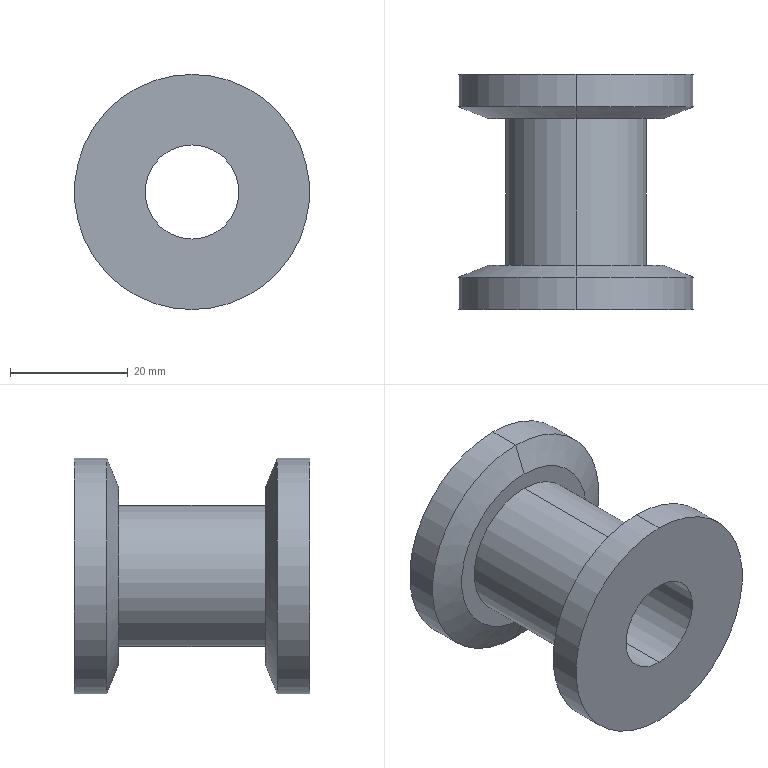Part | SolidWorks | features Chamfer 1, Extrusion 1, RevCut 1 | 1 solid | 16 faces | box 40 x 40 x 40 mm | volume 20965 mm3 | cylinder 8 | cone 4 | plane 4 | commonest cylinder face diameters 40 x4 16 x2 24 x2
STEP:
#1=CARTESIAN_POINT('',(0.,7.5,15.));
#2=VERTEX_POINT('',#1);
#3=CARTESIAN_POINT('',(0.,7.5,-15.));
#4=VERTEX_POINT('',#3);
#5=CARTESIAN_POINT('',(0.,7.5,0.));
#6=DIRECTION('',(0.,1.,0.));
#7=DIRECTION('',(0.,0.,-1.));
#8=AXIS2_PLACEMENT_3D('',#5,#6,#7);
#9=CIRCLE('',#8,15.);
#10=EDGE_CURVE('',#2,#4,#9,.T.);
#11=ORIENTED_EDGE('',*,*,#10,.F.);
#12=CARTESIAN_POINT('',(0.,5.5,20.));
#13=VERTEX_POINT('',#12);
#14=CARTESIAN_POINT('',(0.,5.5,20.));
#15=DIRECTION('',(0.,-0.3714,0.9285));
#16=VECTOR('',#15,1000.);
#17=LINE('',#14,#16);
#18=EDGE_CURVE('',#2,#13,#17,.T.);
#19=ORIENTED_EDGE('',*,*,#18,.T.);
#20=CARTESIAN_POINT('',(0.,5.5,-20.));
#21=VERTEX_POINT('',#20);
#22=CARTESIAN_POINT('',(0.,5.5,0.));
#23=DIRECTION('',(0.,-1.,0.));
#24=DIRECTION('',(0.,0.,-1.));
#25=AXIS2_PLACEMENT_3D('',#22,#23,#24);
#26=CIRCLE('',#25,20.);
#27=EDGE_CURVE('',#21,#13,#26,.T.);
#28=ORIENTED_EDGE('',*,*,#27,.F.);
#29=CARTESIAN_POINT('',(0.,5.5,-20.));
#30=DIRECTION('',(0.,-0.3714,-0.9285));
#31=VECTOR('',#30,1000.);
#32=LINE('',#29,#31);
#33=EDGE_CURVE('',#4,#21,#32,.T.);
#34=ORIENTED_EDGE('',*,*,#33,.F.);
#35=EDGE_LOOP('',(#11,#19,#28,#34));
#36=FACE_OUTER_BOUND('',#35,.T.);
#37=CARTESIAN_POINT('',(0.,5.5,0.));
#38=DIRECTION('',(0.,-1.,0.));
#39=DIRECTION('',(0.,0.,-1.));
#40=AXIS2_PLACEMENT_3D('',#37,#38,#39);
#41=CONICAL_SURFACE('',#40,20.,1.19);
#42=ADVANCED_FACE('',(#36),#41,.T.);
#43=CARTESIAN_POINT('',(0.,32.5,-15.));
#44=VERTEX_POINT('',#43);
#45=CARTESIAN_POINT('',(0.,32.5,15.));
#46=VERTEX_POINT('',#45);
#47=CARTESIAN_POINT('',(0.,32.5,0.));
#48=DIRECTION('',(0.,-1.,0.));
#49=DIRECTION('',(0.,0.,1.));
#50=AXIS2_PLACEMENT_3D('',#47,#48,#49);
#51=CIRCLE('',#50,15.);
#52=EDGE_CURVE('',#44,#46,#51,.T.);
#53=ORIENTED_EDGE('',*,*,#52,.F.);
#54=CARTESIAN_POINT('',(0.,34.5,-20.));
#55=VERTEX_POINT('',#54);
#56=CARTESIAN_POINT('',(0.,34.5,-20.));
#57=DIRECTION('',(0.,0.3714,-0.9285));
#58=VECTOR('',#57,1000.);
#59=LINE('',#56,#58);
#60=EDGE_CURVE('',#44,#55,#59,.T.);
#61=ORIENTED_EDGE('',*,*,#60,.T.);
#62=CARTESIAN_POINT('',(0.,34.5,20.));
#63=VERTEX_POINT('',#62);
#64=CARTESIAN_POINT('',(0.,34.5,0.));
#65=DIRECTION('',(0.,1.,0.));
#66=DIRECTION('',(0.,0.,1.));
#67=AXIS2_PLACEMENT_3D('',#64,#65,#66);
#68=CIRCLE('',#67,20.);
#69=EDGE_CURVE('',#63,#55,#68,.T.);
#70=ORIENTED_EDGE('',*,*,#69,.F.);
#71=CARTESIAN_POINT('',(0.,34.5,20.));
#72=DIRECTION('',(0.,0.3714,0.9285));
#73=VECTOR('',#72,1000.);
#74=LINE('',#71,#73);
#75=EDGE_CURVE('',#46,#63,#74,.T.);
#76=ORIENTED_EDGE('',*,*,#75,.F.);
#77=EDGE_LOOP('',(#53,#61,#70,#76));
#78=FACE_OUTER_BOUND('',#77,.T.);
#79=CARTESIAN_POINT('',(0.,34.5,0.));
#80=DIRECTION('',(0.,1.,0.));
#81=DIRECTION('',(0.,0.,1.));
#82=AXIS2_PLACEMENT_3D('',#79,#80,#81);
#83=CONICAL_SURFACE('',#82,20.,1.19);
#84=ADVANCED_FACE('',(#78),#83,.T.);
#85=CARTESIAN_POINT('',(0.,32.5,-12.));
#86=VERTEX_POINT('',#85);
#87=CARTESIAN_POINT('',(0.,32.5,12.));
#88=VERTEX_POINT('',#87);
#89=CARTESIAN_POINT('',(0.,32.5,0.));
#90=DIRECTION('',(0.,-1.,0.));
#91=DIRECTION('',(0.,0.,-1.));
#92=AXIS2_PLACEMENT_3D('',#89,#90,#91);
#93=CIRCLE('',#92,12.);
#94=EDGE_CURVE('',#86,#88,#93,.T.);
#95=ORIENTED_EDGE('',*,*,#94,.T.);
#96=CARTESIAN_POINT('',(0.,7.5,12.));
#97=VERTEX_POINT('',#96);
#98=CARTESIAN_POINT('',(0.,0.,12.));
#99=DIRECTION('',(0.,-1.,0.));
#100=VECTOR('',#99,1000.);
#101=LINE('',#98,#100);
#102=EDGE_CURVE('',#88,#97,#101,.T.);
#103=ORIENTED_EDGE('',*,*,#102,.T.);
#104=CARTESIAN_POINT('',(0.,7.5,-12.));
#105=VERTEX_POINT('',#104);
#106=CARTESIAN_POINT('',(0.,7.5,0.));
#107=DIRECTION('',(0.,-1.,0.));
#108=DIRECTION('',(0.,0.,-1.));
#109=AXIS2_PLACEMENT_3D('',#106,#107,#108);
#110=CIRCLE('',#109,12.);
#111=EDGE_CURVE('',#105,#97,#110,.T.);
#112=ORIENTED_EDGE('',*,*,#111,.F.);
#113=CARTESIAN_POINT('',(0.,0.,-12.));
#114=DIRECTION('',(0.,-1.,0.));
#115=VECTOR('',#114,1000.);
#116=LINE('',#113,#115);
#117=EDGE_CURVE('',#86,#105,#116,.T.);
#118=ORIENTED_EDGE('',*,*,#117,.F.);
#119=EDGE_LOOP('',(#95,#103,#112,#118));
#120=FACE_OUTER_BOUND('',#119,.T.);
#121=CARTESIAN_POINT('',(0.,0.,0.));
#122=DIRECTION('',(0.,-1.,0.));
#123=DIRECTION('',(0.,0.,-1.));
#124=AXIS2_PLACEMENT_3D('',#121,#122,#123);
#125=CYLINDRICAL_SURFACE('',#124,12.);
#126=ADVANCED_FACE('',(#120),#125,.T.);
#127=CARTESIAN_POINT('',(0.,40.,-8.));
#128=VERTEX_POINT('',#127);
#129=CARTESIAN_POINT('',(0.,40.,8.));
#130=VERTEX_POINT('',#129);
#131=CARTESIAN_POINT('',(0.,40.,0.));
#132=DIRECTION('',(0.,1.,0.));
#133=DIRECTION('',(0.,0.,1.));
#134=AXIS2_PLACEMENT_3D('',#131,#132,#133);
#135=CIRCLE('',#134,8.);
#136=EDGE_CURVE('',#128,#130,#135,.T.);
#137=ORIENTED_EDGE('',*,*,#136,.T.);
#138=CARTESIAN_POINT('',(0.,0.,8.));
#139=VERTEX_POINT('',#138);
#140=CARTESIAN_POINT('',(0.,40.,8.));
#141=DIRECTION('',(0.,-1.,0.));
#142=VECTOR('',#141,1000.);
#143=LINE('',#140,#142);
#144=EDGE_CURVE('',#130,#139,#143,.T.);
#145=ORIENTED_EDGE('',*,*,#144,.T.);
#146=CARTESIAN_POINT('',(0.,0.,-8.));
#147=VERTEX_POINT('',#146);
#148=CARTESIAN_POINT('',(0.,0.,0.));
#149=DIRECTION('',(0.,1.,0.));
#150=DIRECTION('',(0.,0.,1.));
#151=AXIS2_PLACEMENT_3D('',#148,#149,#150);
#152=CIRCLE('',#151,8.);
#153=EDGE_CURVE('',#147,#139,#152,.T.);
#154=ORIENTED_EDGE('',*,*,#153,.F.);
#155=CARTESIAN_POINT('',(0.,40.,-8.));
#156=DIRECTION('',(0.,-1.,0.));
#157=VECTOR('',#156,1000.);
#158=LINE('',#155,#157);
#159=EDGE_CURVE('',#128,#147,#158,.T.);
#160=ORIENTED_EDGE('',*,*,#159,.F.);
#161=EDGE_LOOP('',(#137,#145,#154,#160));
#162=FACE_OUTER_BOUND('',#161,.T.);
#163=CARTESIAN_POINT('',(0.,40.,0.));
#164=DIRECTION('',(0.,-1.,0.));
#165=DIRECTION('',(0.,0.,-1.));
#166=AXIS2_PLACEMENT_3D('',#163,#164,#165);
#167=CYLINDRICAL_SURFACE('',#166,8.);
#168=ADVANCED_FACE('',(#162),#167,.F.);
#169=CARTESIAN_POINT('',(0.,40.,20.));
#170=VERTEX_POINT('',#169);
#171=CARTESIAN_POINT('',(0.,40.,-20.));
#172=VERTEX_POINT('',#171);
#173=CARTESIAN_POINT('',(0.,40.,0.));
#174=DIRECTION('',(0.,1.,0.));
#175=DIRECTION('',(0.,0.,1.));
#176=AXIS2_PLACEMENT_3D('',#173,#174,#175);
#177=CIRCLE('',#176,20.);
#178=EDGE_CURVE('',#170,#172,#177,.T.);
#179=ORIENTED_EDGE('',*,*,#178,.F.);
#180=CARTESIAN_POINT('',(0.,40.,20.));
#181=DIRECTION('',(0.,-1.,0.));
#182=VECTOR('',#181,1000.);
#183=LINE('',#180,#182);
#184=EDGE_CURVE('',#170,#63,#183,.T.);
#185=ORIENTED_EDGE('',*,*,#184,.T.);
#186=ORIENTED_EDGE('',*,*,#69,.T.);
#187=CARTESIAN_POINT('',(0.,40.,-20.));
#188=DIRECTION('',(0.,-1.,0.));
#189=VECTOR('',#188,1000.);
#190=LINE('',#187,#189);
#191=EDGE_CURVE('',#172,#55,#190,.T.);
#192=ORIENTED_EDGE('',*,*,#191,.F.);
#193=EDGE_LOOP('',(#179,#185,#186,#192));
#194=FACE_OUTER_BOUND('',#193,.T.);
#195=CARTESIAN_POINT('',(0.,40.,0.));
#196=DIRECTION('',(0.,-1.,0.));
#197=DIRECTION('',(0.,0.,-1.));
#198=AXIS2_PLACEMENT_3D('',#195,#196,#197);
#199=CYLINDRICAL_SURFACE('',#198,20.);
#200=ADVANCED_FACE('',(#194),#199,.T.);
#201=ORIENTED_EDGE('',*,*,#27,.T.);
#202=CARTESIAN_POINT('',(0.,0.,20.));
#203=VERTEX_POINT('',#202);
#204=CARTESIAN_POINT('',(0.,40.,20.));
#205=DIRECTION('',(0.,-1.,0.));
#206=VECTOR('',#205,1000.);
#207=LINE('',#204,#206);
#208=EDGE_CURVE('',#13,#203,#207,.T.);
#209=ORIENTED_EDGE('',*,*,#208,.T.);
#210=CARTESIAN_POINT('',(0.,0.,-20.));
#211=VERTEX_POINT('',#210);
#212=CARTESIAN_POINT('',(0.,0.,0.));
#213=DIRECTION('',(0.,1.,0.));
#214=DIRECTION('',(0.,0.,1.));
#215=AXIS2_PLACEMENT_3D('',#212,#213,#214);
#216=CIRCLE('',#215,20.);
#217=EDGE_CURVE('',#203,#211,#216,.T.);
#218=ORIENTED_EDGE('',*,*,#217,.T.);
#219=CARTESIAN_POINT('',(0.,40.,-20.));
#220=DIRECTION('',(0.,-1.,0.));
#221=VECTOR('',#220,1000.);
#222=LINE('',#219,#221);
#223=EDGE_CURVE('',#21,#211,#222,.T.);
#224=ORIENTED_EDGE('',*,*,#223,.F.);
#225=EDGE_LOOP('',(#201,#209,#218,#224));
#226=FACE_OUTER_BOUND('',#225,.T.);
#227=CARTESIAN_POINT('',(0.,40.,0.));
#228=DIRECTION('',(0.,-1.,0.));
#229=DIRECTION('',(0.,0.,-1.));
#230=AXIS2_PLACEMENT_3D('',#227,#228,#229);
#231=CYLINDRICAL_SURFACE('',#230,20.);
#232=ADVANCED_FACE('',(#226),#231,.T.);
#233=ORIENTED_EDGE('',*,*,#208,.F.);
#234=CARTESIAN_POINT('',(0.,5.5,0.));
#235=DIRECTION('',(0.,-1.,0.));
#236=DIRECTION('',(0.,0.,-1.));
#237=AXIS2_PLACEMENT_3D('',#234,#235,#236);
#238=CIRCLE('',#237,20.);
#239=EDGE_CURVE('',#13,#21,#238,.T.);
#240=ORIENTED_EDGE('',*,*,#239,.T.);
#241=ORIENTED_EDGE('',*,*,#223,.T.);
#242=CARTESIAN_POINT('',(0.,0.,0.));
#243=DIRECTION('',(0.,1.,0.));
#244=DIRECTION('',(0.,0.,1.));
#245=AXIS2_PLACEMENT_3D('',#242,#243,#244);
#246=CIRCLE('',#245,20.);
#247=EDGE_CURVE('',#211,#203,#246,.T.);
#248=ORIENTED_EDGE('',*,*,#247,.T.);
#249=EDGE_LOOP('',(#233,#240,#241,#248));
#250=FACE_OUTER_BOUND('',#249,.T.);
#251=CARTESIAN_POINT('',(0.,40.,0.));
#252=DIRECTION('',(0.,-1.,0.));
#253=DIRECTION('',(0.,0.,-1.));
#254=AXIS2_PLACEMENT_3D('',#251,#252,#253);
#255=CYLINDRICAL_SURFACE('',#254,20.);
#256=ADVANCED_FACE('',(#250),#255,.T.);
#257=CARTESIAN_POINT('',(0.,40.,0.));
#258=DIRECTION('',(0.,1.,0.));
#259=DIRECTION('',(0.,0.,1.));
#260=AXIS2_PLACEMENT_3D('',#257,#258,#259);
#261=CIRCLE('',#260,20.);
#262=EDGE_CURVE('',#172,#170,#261,.T.);
#263=ORIENTED_EDGE('',*,*,#262,.T.);
#264=ORIENTED_EDGE('',*,*,#178,.T.);
#265=EDGE_LOOP('',(#263,#264));
#266=FACE_OUTER_BOUND('',#265,.T.);
#267=ORIENTED_EDGE('',*,*,#136,.F.);
#268=CARTESIAN_POINT('',(0.,40.,0.));
#269=DIRECTION('',(0.,1.,0.));
#270=DIRECTION('',(0.,0.,1.));
#271=AXIS2_PLACEMENT_3D('',#268,#269,#270);
#272=CIRCLE('',#271,8.);
#273=EDGE_CURVE('',#130,#128,#272,.T.);
#274=ORIENTED_EDGE('',*,*,#273,.F.);
#275=EDGE_LOOP('',(#267,#274));
#276=FACE_BOUND('',#275,.T.);
#277=CARTESIAN_POINT('',(0.,40.,0.));
#278=DIRECTION('',(0.,1.,0.));
#279=DIRECTION('',(0.,0.,1.));
#280=AXIS2_PLACEMENT_3D('',#277,#278,#279);
#281=PLANE('',#280);
#282=ADVANCED_FACE('',(#266,#276),#281,.T.);
#283=ORIENTED_EDGE('',*,*,#247,.F.);
#284=ORIENTED_EDGE('',*,*,#217,.F.);
#285=EDGE_LOOP('',(#283,#284));
#286=FACE_OUTER_BOUND('',#285,.T.);
#287=ORIENTED_EDGE('',*,*,#153,.T.);
#288=CARTESIAN_POINT('',(0.,0.,0.));
#289=DIRECTION('',(0.,1.,0.));
#290=DIRECTION('',(0.,0.,1.));
#291=AXIS2_PLACEMENT_3D('',#288,#289,#290);
#292=CIRCLE('',#291,8.);
#293=EDGE_CURVE('',#139,#147,#292,.T.);
#294=ORIENTED_EDGE('',*,*,#293,.T.);
#295=EDGE_LOOP('',(#287,#294));
#296=FACE_BOUND('',#295,.T.);
#297=CARTESIAN_POINT('',(0.,0.,0.));
#298=DIRECTION('',(0.,1.,0.));
#299=DIRECTION('',(0.,0.,1.));
#300=AXIS2_PLACEMENT_3D('',#297,#298,#299);
#301=PLANE('',#300);
#302=ADVANCED_FACE('',(#286,#296),#301,.F.);
#303=ORIENTED_EDGE('',*,*,#184,.F.);
#304=ORIENTED_EDGE('',*,*,#262,.F.);
#305=ORIENTED_EDGE('',*,*,#191,.T.);
#306=CARTESIAN_POINT('',(0.,34.5,0.));
#307=DIRECTION('',(0.,1.,0.));
#308=DIRECTION('',(0.,0.,1.));
#309=AXIS2_PLACEMENT_3D('',#306,#307,#308);
#310=CIRCLE('',#309,20.);
#311=EDGE_CURVE('',#55,#63,#310,.T.);
#312=ORIENTED_EDGE('',*,*,#311,.T.);
#313=EDGE_LOOP('',(#303,#304,#305,#312));
#314=FACE_OUTER_BOUND('',#313,.T.);
#315=CARTESIAN_POINT('',(0.,40.,0.));
#316=DIRECTION('',(0.,-1.,0.));
#317=DIRECTION('',(0.,0.,-1.));
#318=AXIS2_PLACEMENT_3D('',#315,#316,#317);
#319=CYLINDRICAL_SURFACE('',#318,20.);
#320=ADVANCED_FACE('',(#314),#319,.T.);
#321=ORIENTED_EDGE('',*,*,#144,.F.);
#322=ORIENTED_EDGE('',*,*,#273,.T.);
#323=ORIENTED_EDGE('',*,*,#159,.T.);
#324=ORIENTED_EDGE('',*,*,#293,.F.);
#325=EDGE_LOOP('',(#321,#322,#323,#324));
#326=FACE_OUTER_BOUND('',#325,.T.);
#327=CARTESIAN_POINT('',(0.,40.,0.));
#328=DIRECTION('',(0.,-1.,0.));
#329=DIRECTION('',(0.,0.,-1.));
#330=AXIS2_PLACEMENT_3D('',#327,#328,#329);
#331=CYLINDRICAL_SURFACE('',#330,8.);
#332=ADVANCED_FACE('',(#326),#331,.F.);
#333=CARTESIAN_POINT('',(0.,7.5,0.));
#334=DIRECTION('',(0.,1.,0.));
#335=DIRECTION('',(0.,0.,-1.));
#336=AXIS2_PLACEMENT_3D('',#333,#334,#335);
#337=CIRCLE('',#336,15.);
#338=EDGE_CURVE('',#4,#2,#337,.T.);
#339=ORIENTED_EDGE('',*,*,#338,.T.);
#340=ORIENTED_EDGE('',*,*,#10,.T.);
#341=EDGE_LOOP('',(#339,#340));
#342=FACE_OUTER_BOUND('',#341,.T.);
#343=ORIENTED_EDGE('',*,*,#111,.T.);
#344=CARTESIAN_POINT('',(0.,7.5,0.));
#345=DIRECTION('',(0.,-1.,0.));
#346=DIRECTION('',(0.,0.,-1.));
#347=AXIS2_PLACEMENT_3D('',#344,#345,#346);
#348=CIRCLE('',#347,12.);
#349=EDGE_CURVE('',#97,#105,#348,.T.);
#350=ORIENTED_EDGE('',*,*,#349,.T.);
#351=EDGE_LOOP('',(#343,#350));
#352=FACE_BOUND('',#351,.T.);
#353=CARTESIAN_POINT('',(28.,7.5,0.));
#354=DIRECTION('',(0.,-1.,0.));
#355=DIRECTION('',(0.,0.,-1.));
#356=AXIS2_PLACEMENT_3D('',#353,#354,#355);
#357=PLANE('',#356);
#358=ADVANCED_FACE('',(#342,#352),#357,.F.);
#359=CARTESIAN_POINT('',(0.,32.5,0.));
#360=DIRECTION('',(0.,-1.,0.));
#361=DIRECTION('',(0.,0.,1.));
#362=AXIS2_PLACEMENT_3D('',#359,#360,#361);
#363=CIRCLE('',#362,15.);
#364=EDGE_CURVE('',#46,#44,#363,.T.);
#365=ORIENTED_EDGE('',*,*,#364,.T.);
#366=ORIENTED_EDGE('',*,*,#52,.T.);
#367=EDGE_LOOP('',(#365,#366));
#368=FACE_OUTER_BOUND('',#367,.T.);
#369=ORIENTED_EDGE('',*,*,#94,.F.);
#370=CARTESIAN_POINT('',(0.,32.5,0.));
#371=DIRECTION('',(0.,-1.,0.));
#372=DIRECTION('',(0.,0.,-1.));
#373=AXIS2_PLACEMENT_3D('',#370,#371,#372);
#374=CIRCLE('',#373,12.);
#375=EDGE_CURVE('',#88,#86,#374,.T.);
#376=ORIENTED_EDGE('',*,*,#375,.F.);
#377=EDGE_LOOP('',(#369,#376));
#378=FACE_BOUND('',#377,.T.);
#379=CARTESIAN_POINT('',(28.,32.5,0.));
#380=DIRECTION('',(0.,1.,0.));
#381=DIRECTION('',(0.,0.,1.));
#382=AXIS2_PLACEMENT_3D('',#379,#380,#381);
#383=PLANE('',#382);
#384=ADVANCED_FACE('',(#368,#378),#383,.F.);
#385=ORIENTED_EDGE('',*,*,#102,.F.);
#386=ORIENTED_EDGE('',*,*,#375,.T.);
#387=ORIENTED_EDGE('',*,*,#117,.T.);
#388=ORIENTED_EDGE('',*,*,#349,.F.);
#389=EDGE_LOOP('',(#385,#386,#387,#388));
#390=FACE_OUTER_BOUND('',#389,.T.);
#391=CARTESIAN_POINT('',(0.,0.,0.));
#392=DIRECTION('',(0.,-1.,0.));
#393=DIRECTION('',(0.,0.,-1.));
#394=AXIS2_PLACEMENT_3D('',#391,#392,#393);
#395=CYLINDRICAL_SURFACE('',#394,12.);
#396=ADVANCED_FACE('',(#390),#395,.T.);
#397=ORIENTED_EDGE('',*,*,#60,.F.);
#398=ORIENTED_EDGE('',*,*,#364,.F.);
#399=ORIENTED_EDGE('',*,*,#75,.T.);
#400=ORIENTED_EDGE('',*,*,#311,.F.);
#401=EDGE_LOOP('',(#397,#398,#399,#400));
#402=FACE_OUTER_BOUND('',#401,.T.);
#403=CARTESIAN_POINT('',(0.,34.5,0.));
#404=DIRECTION('',(0.,1.,0.));
#405=DIRECTION('',(0.,0.,1.));
#406=AXIS2_PLACEMENT_3D('',#403,#404,#405);
#407=CONICAL_SURFACE('',#406,20.,1.19);
#408=ADVANCED_FACE('',(#402),#407,.T.);
#409=ORIENTED_EDGE('',*,*,#18,.F.);
#410=ORIENTED_EDGE('',*,*,#338,.F.);
#411=ORIENTED_EDGE('',*,*,#33,.T.);
#412=ORIENTED_EDGE('',*,*,#239,.F.);
#413=EDGE_LOOP('',(#409,#410,#411,#412));
#414=FACE_OUTER_BOUND('',#413,.T.);
#415=CARTESIAN_POINT('',(0.,5.5,0.));
#416=DIRECTION('',(0.,-1.,0.));
#417=DIRECTION('',(0.,0.,-1.));
#418=AXIS2_PLACEMENT_3D('',#415,#416,#417);
#419=CONICAL_SURFACE('',#418,20.,1.19);
#420=ADVANCED_FACE('',(#414),#419,.T.);
#421=CLOSED_SHELL('',(#42,#84,#126,#168,#200,#232,#256,#282,#302,#320,#332,#358,#384,#396,#408,#420));
#422=MANIFOLD_SOLID_BREP('',#421);
#423=CARTESIAN_POINT('',(0.,0.,0.));
#424=DIRECTION('',(0.,0.,1.));
#425=DIRECTION('',(1.,0.,0.));
#426=AXIS2_PLACEMENT_3D('',#423,#424,#425);
#427=(LENGTH_UNIT()NAMED_UNIT(*)SI_UNIT(.MILLI.,.METRE.));
#428=UNCERTAINTY_MEASURE_WITH_UNIT(LENGTH_MEASURE(0.00001),#427,'','');
#429=(NAMED_UNIT(*)PLANE_ANGLE_UNIT()SI_UNIT($,.RADIAN.));
#430=(NAMED_UNIT(*)SI_UNIT($,.STERADIAN.)SOLID_ANGLE_UNIT());
#431=(GEOMETRIC_REPRESENTATION_CONTEXT(3)GLOBAL_UNCERTAINTY_ASSIGNED_CONTEXT((#428))GLOBAL_UNIT_ASSIGNED_CONTEXT((#427,#429,#430))REPRESENTATION_CONTEXT('',''));
#432=ADVANCED_BREP_SHAPE_REPRESENTATION('',(#422,#426),#431);